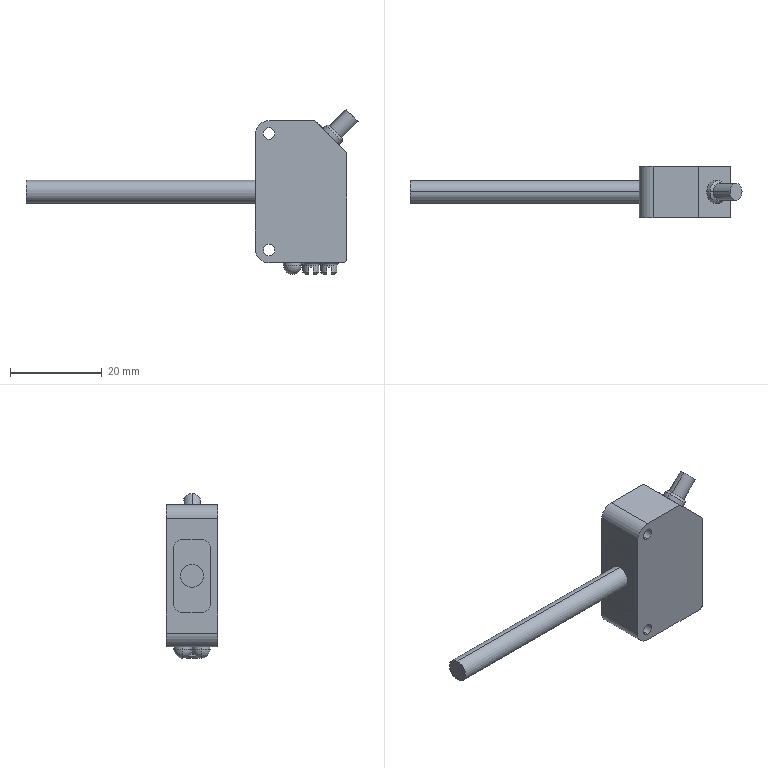Part | SolidWorks | features Boss 4, Chamfer 3, Fillet 3, Cut 2, Dome 2, Extrusion 1, HoleWzd 1, ICE 1 | 1 solid | 66 faces | box 72.394 x 11.2 x 35.904 mm | volume 7657 mm3 | cylinder 25 | plane 25 | cone 8 | torus 4 | sphere 4 | commonest cylinder face diameters 2.5 x4 3.5 x4 3.9 x4 4 x4 5 x4 3.7 x2